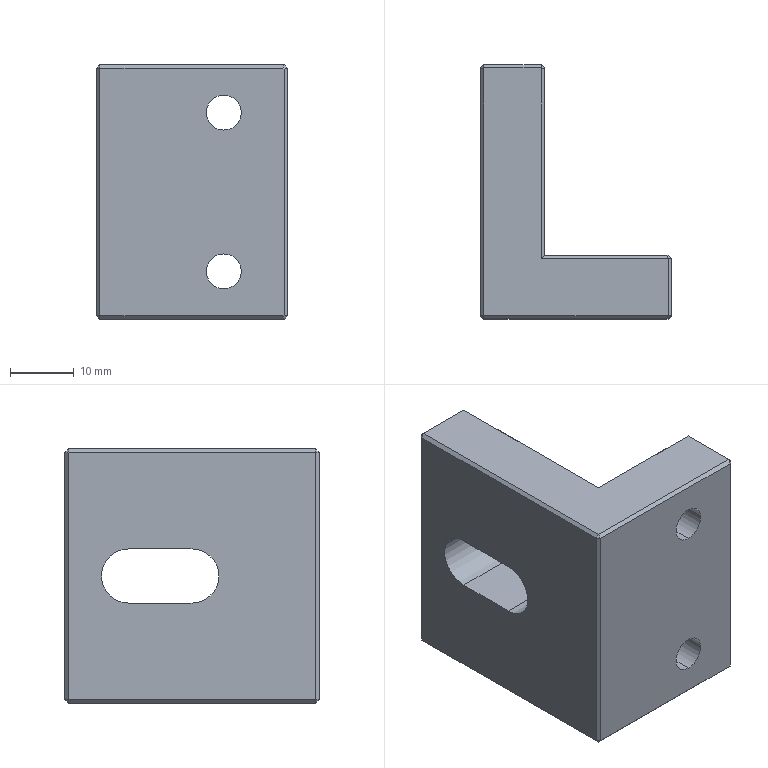Part | SolidWorks | features Chamfer 3, ICE 2, Extrusion 1, HoleWzd 1 | 1 solid | 49 faces | box 30 x 40 x 40 mm | volume 21456 mm3 | plane 39 | cylinder 10 | commonest cylinder face diameters 5.5 x4 10 x4 8.5 x2
STEP:
#1=CARTESIAN_POINT('',(5.,4.6,7.5));
#2=VERTEX_POINT('',#1);
#3=CARTESIAN_POINT('',(5.,4.6,17.5));
#4=VERTEX_POINT('',#3);
#5=CARTESIAN_POINT('',(5.,4.6,12.5));
#6=DIRECTION('',(0.,1.,0.));
#7=DIRECTION('',(0.,0.,1.));
#8=AXIS2_PLACEMENT_3D('',#5,#6,#7);
#9=CIRCLE('',#8,5.);
#10=EDGE_CURVE('',#2,#4,#9,.T.);
#11=ORIENTED_EDGE('',*,*,#10,.F.);
#12=CARTESIAN_POINT('',(5.,10.,7.5));
#13=VERTEX_POINT('',#12);
#14=CARTESIAN_POINT('',(5.,10.,7.5));
#15=DIRECTION('',(0.,1.,0.));
#16=VECTOR('',#15,1000.);
#17=LINE('',#14,#16);
#18=EDGE_CURVE('',#2,#13,#17,.T.);
#19=ORIENTED_EDGE('',*,*,#18,.T.);
#20=CARTESIAN_POINT('',(5.,10.,17.5));
#21=VERTEX_POINT('',#20);
#22=CARTESIAN_POINT('',(5.,10.,12.5));
#23=DIRECTION('',(0.,1.,0.));
#24=DIRECTION('',(0.,0.,1.));
#25=AXIS2_PLACEMENT_3D('',#22,#23,#24);
#26=CIRCLE('',#25,5.);
#27=EDGE_CURVE('',#13,#21,#26,.T.);
#28=ORIENTED_EDGE('',*,*,#27,.T.);
#29=CARTESIAN_POINT('',(5.,10.,17.5));
#30=DIRECTION('',(0.,1.,0.));
#31=VECTOR('',#30,1000.);
#32=LINE('',#29,#31);
#33=EDGE_CURVE('',#4,#21,#32,.T.);
#34=ORIENTED_EDGE('',*,*,#33,.F.);
#35=EDGE_LOOP('',(#11,#19,#28,#34));
#36=FACE_OUTER_BOUND('',#35,.T.);
#37=CARTESIAN_POINT('',(5.,10.,12.5));
#38=DIRECTION('',(0.,1.,0.));
#39=DIRECTION('',(0.,0.,1.));
#40=AXIS2_PLACEMENT_3D('',#37,#38,#39);
#41=CYLINDRICAL_SURFACE('',#40,5.);
#42=ADVANCED_FACE('',(#36),#41,.F.);
#43=CARTESIAN_POINT('',(5.,0.,9.75));
#44=VERTEX_POINT('',#43);
#45=CARTESIAN_POINT('',(5.,0.,15.25));
#46=VERTEX_POINT('',#45);
#47=CARTESIAN_POINT('',(5.,0.,12.5));
#48=DIRECTION('',(0.,1.,0.));
#49=DIRECTION('',(0.,0.,1.));
#50=AXIS2_PLACEMENT_3D('',#47,#48,#49);
#51=CIRCLE('',#50,2.75);
#52=EDGE_CURVE('',#44,#46,#51,.T.);
#53=ORIENTED_EDGE('',*,*,#52,.F.);
#54=CARTESIAN_POINT('',(5.,4.6,9.75));
#55=VERTEX_POINT('',#54);
#56=CARTESIAN_POINT('',(5.,10.,9.75));
#57=DIRECTION('',(0.,1.,0.));
#58=VECTOR('',#57,1000.);
#59=LINE('',#56,#58);
#60=EDGE_CURVE('',#44,#55,#59,.T.);
#61=ORIENTED_EDGE('',*,*,#60,.T.);
#62=CARTESIAN_POINT('',(5.,4.6,15.25));
#63=VERTEX_POINT('',#62);
#64=CARTESIAN_POINT('',(5.,4.6,12.5));
#65=DIRECTION('',(0.,1.,0.));
#66=DIRECTION('',(0.,0.,1.));
#67=AXIS2_PLACEMENT_3D('',#64,#65,#66);
#68=CIRCLE('',#67,2.75);
#69=EDGE_CURVE('',#55,#63,#68,.T.);
#70=ORIENTED_EDGE('',*,*,#69,.T.);
#71=CARTESIAN_POINT('',(5.,10.,15.25));
#72=DIRECTION('',(0.,1.,0.));
#73=VECTOR('',#72,1000.);
#74=LINE('',#71,#73);
#75=EDGE_CURVE('',#46,#63,#74,.T.);
#76=ORIENTED_EDGE('',*,*,#75,.F.);
#77=EDGE_LOOP('',(#53,#61,#70,#76));
#78=FACE_OUTER_BOUND('',#77,.T.);
#79=CARTESIAN_POINT('',(5.,10.,12.5));
#80=DIRECTION('',(0.,1.,0.));
#81=DIRECTION('',(0.,0.,1.));
#82=AXIS2_PLACEMENT_3D('',#79,#80,#81);
#83=CYLINDRICAL_SURFACE('',#82,2.75);
#84=ADVANCED_FACE('',(#78),#83,.F.);
#85=CARTESIAN_POINT('',(5.,4.6,-17.5));
#86=VERTEX_POINT('',#85);
#87=CARTESIAN_POINT('',(5.,4.6,-7.5));
#88=VERTEX_POINT('',#87);
#89=CARTESIAN_POINT('',(5.,4.6,-12.5));
#90=DIRECTION('',(0.,1.,0.));
#91=DIRECTION('',(0.,0.,1.));
#92=AXIS2_PLACEMENT_3D('',#89,#90,#91);
#93=CIRCLE('',#92,5.);
#94=EDGE_CURVE('',#86,#88,#93,.T.);
#95=ORIENTED_EDGE('',*,*,#94,.F.);
#96=CARTESIAN_POINT('',(5.,10.,-17.5));
#97=VERTEX_POINT('',#96);
#98=CARTESIAN_POINT('',(5.,10.,-17.5));
#99=DIRECTION('',(0.,1.,0.));
#100=VECTOR('',#99,1000.);
#101=LINE('',#98,#100);
#102=EDGE_CURVE('',#86,#97,#101,.T.);
#103=ORIENTED_EDGE('',*,*,#102,.T.);
#104=CARTESIAN_POINT('',(5.,10.,-7.5));
#105=VERTEX_POINT('',#104);
#106=CARTESIAN_POINT('',(5.,10.,-12.5));
#107=DIRECTION('',(0.,1.,0.));
#108=DIRECTION('',(0.,0.,1.));
#109=AXIS2_PLACEMENT_3D('',#106,#107,#108);
#110=CIRCLE('',#109,5.);
#111=EDGE_CURVE('',#97,#105,#110,.T.);
#112=ORIENTED_EDGE('',*,*,#111,.T.);
#113=CARTESIAN_POINT('',(5.,10.,-7.5));
#114=DIRECTION('',(0.,1.,0.));
#115=VECTOR('',#114,1000.);
#116=LINE('',#113,#115);
#117=EDGE_CURVE('',#88,#105,#116,.T.);
#118=ORIENTED_EDGE('',*,*,#117,.F.);
#119=EDGE_LOOP('',(#95,#103,#112,#118));
#120=FACE_OUTER_BOUND('',#119,.T.);
#121=CARTESIAN_POINT('',(5.,10.,-12.5));
#122=DIRECTION('',(0.,1.,0.));
#123=DIRECTION('',(0.,0.,1.));
#124=AXIS2_PLACEMENT_3D('',#121,#122,#123);
#125=CYLINDRICAL_SURFACE('',#124,5.);
#126=ADVANCED_FACE('',(#120),#125,.F.);
#127=CARTESIAN_POINT('',(5.,0.,-15.25));
#128=VERTEX_POINT('',#127);
#129=CARTESIAN_POINT('',(5.,0.,-9.75));
#130=VERTEX_POINT('',#129);
#131=CARTESIAN_POINT('',(5.,0.,-12.5));
#132=DIRECTION('',(0.,1.,0.));
#133=DIRECTION('',(0.,0.,1.));
#134=AXIS2_PLACEMENT_3D('',#131,#132,#133);
#135=CIRCLE('',#134,2.75);
#136=EDGE_CURVE('',#128,#130,#135,.T.);
#137=ORIENTED_EDGE('',*,*,#136,.F.);
#138=CARTESIAN_POINT('',(5.,4.6,-15.25));
#139=VERTEX_POINT('',#138);
#140=CARTESIAN_POINT('',(5.,10.,-15.25));
#141=DIRECTION('',(0.,1.,0.));
#142=VECTOR('',#141,1000.);
#143=LINE('',#140,#142);
#144=EDGE_CURVE('',#128,#139,#143,.T.);
#145=ORIENTED_EDGE('',*,*,#144,.T.);
#146=CARTESIAN_POINT('',(5.,4.6,-9.75));
#147=VERTEX_POINT('',#146);
#148=CARTESIAN_POINT('',(5.,4.6,-12.5));
#149=DIRECTION('',(0.,1.,0.));
#150=DIRECTION('',(0.,0.,1.));
#151=AXIS2_PLACEMENT_3D('',#148,#149,#150);
#152=CIRCLE('',#151,2.75);
#153=EDGE_CURVE('',#139,#147,#152,.T.);
#154=ORIENTED_EDGE('',*,*,#153,.T.);
#155=CARTESIAN_POINT('',(5.,10.,-9.75));
#156=DIRECTION('',(0.,1.,0.));
#157=VECTOR('',#156,1000.);
#158=LINE('',#155,#157);
#159=EDGE_CURVE('',#130,#147,#158,.T.);
#160=ORIENTED_EDGE('',*,*,#159,.F.);
#161=EDGE_LOOP('',(#137,#145,#154,#160));
#162=FACE_OUTER_BOUND('',#161,.T.);
#163=CARTESIAN_POINT('',(5.,10.,-12.5));
#164=DIRECTION('',(0.,1.,0.));
#165=DIRECTION('',(0.,0.,1.));
#166=AXIS2_PLACEMENT_3D('',#163,#164,#165);
#167=CYLINDRICAL_SURFACE('',#166,2.75);
#168=ADVANCED_FACE('',(#162),#167,.F.);
#169=CARTESIAN_POINT('',(15.,9.5,19.5));
#170=VERTEX_POINT('',#169);
#171=CARTESIAN_POINT('',(15.,0.5,19.5));
#172=VERTEX_POINT('',#171);
#173=CARTESIAN_POINT('',(15.,10.,19.5));
#174=DIRECTION('',(0.,-1.,0.));
#175=VECTOR('',#174,1000.);
#176=LINE('',#173,#175);
#177=EDGE_CURVE('',#170,#172,#176,.T.);
#178=ORIENTED_EDGE('',*,*,#177,.T.);
#179=CARTESIAN_POINT('',(15.,0.5,-19.5));
#180=VERTEX_POINT('',#179);
#181=CARTESIAN_POINT('',(15.,0.5,-20.));
#182=DIRECTION('',(0.,0.,-1.));
#183=VECTOR('',#182,1000.);
#184=LINE('',#181,#183);
#185=EDGE_CURVE('',#172,#180,#184,.T.);
#186=ORIENTED_EDGE('',*,*,#185,.T.);
#187=CARTESIAN_POINT('',(15.,9.5,-19.5));
#188=VERTEX_POINT('',#187);
#189=CARTESIAN_POINT('',(15.,10.,-19.5));
#190=DIRECTION('',(0.,1.,0.));
#191=VECTOR('',#190,1000.);
#192=LINE('',#189,#191);
#193=EDGE_CURVE('',#180,#188,#192,.T.);
#194=ORIENTED_EDGE('',*,*,#193,.T.);
#195=CARTESIAN_POINT('',(15.,9.5,19.5));
#196=DIRECTION('',(0.,0.,1.));
#197=VECTOR('',#196,1000.);
#198=LINE('',#195,#197);
#199=EDGE_CURVE('',#188,#170,#198,.T.);
#200=ORIENTED_EDGE('',*,*,#199,.T.);
#201=EDGE_LOOP('',(#178,#186,#194,#200));
#202=FACE_OUTER_BOUND('',#201,.T.);
#203=CARTESIAN_POINT('',(15.,10.,-20.));
#204=DIRECTION('',(-1.,0.,0.));
#205=DIRECTION('',(0.,0.,1.));
#206=AXIS2_PLACEMENT_3D('',#203,#204,#205);
#207=PLANE('',#206);
#208=ADVANCED_FACE('',(#202),#207,.F.);
#209=CARTESIAN_POINT('',(14.5,0.5,-20.));
#210=VERTEX_POINT('',#209);
#211=CARTESIAN_POINT('',(-14.5,0.5,-20.));
#212=VERTEX_POINT('',#211);
#213=CARTESIAN_POINT('',(-15.,0.5,-20.));
#214=DIRECTION('',(-1.,0.,0.));
#215=VECTOR('',#214,1000.);
#216=LINE('',#213,#215);
#217=EDGE_CURVE('',#210,#212,#216,.T.);
#218=ORIENTED_EDGE('',*,*,#217,.T.);
#219=CARTESIAN_POINT('',(-14.5,39.5,-20.));
#220=VERTEX_POINT('',#219);
#221=CARTESIAN_POINT('',(-14.5,10.,-20.));
#222=DIRECTION('',(0.,1.,0.));
#223=VECTOR('',#222,1000.);
#224=LINE('',#221,#223);
#225=EDGE_CURVE('',#212,#220,#224,.T.);
#226=ORIENTED_EDGE('',*,*,#225,.T.);
#227=CARTESIAN_POINT('',(-5.5,39.5,-20.));
#228=VERTEX_POINT('',#227);
#229=CARTESIAN_POINT('',(-5.,39.5,-20.));
#230=DIRECTION('',(1.,0.,0.));
#231=VECTOR('',#230,1000.);
#232=LINE('',#229,#231);
#233=EDGE_CURVE('',#220,#228,#232,.T.);
#234=ORIENTED_EDGE('',*,*,#233,.T.);
#235=CARTESIAN_POINT('',(-5.5,9.5,-20.));
#236=VERTEX_POINT('',#235);
#237=CARTESIAN_POINT('',(-5.5,10.,-20.));
#238=DIRECTION('',(0.,-1.,0.));
#239=VECTOR('',#238,1000.);
#240=LINE('',#237,#239);
#241=EDGE_CURVE('',#228,#236,#240,.T.);
#242=ORIENTED_EDGE('',*,*,#241,.T.);
#243=CARTESIAN_POINT('',(14.5,9.5,-20.));
#244=VERTEX_POINT('',#243);
#245=CARTESIAN_POINT('',(14.5,9.5,-20.));
#246=DIRECTION('',(1.,0.,0.));
#247=VECTOR('',#246,1000.);
#248=LINE('',#245,#247);
#249=EDGE_CURVE('',#236,#244,#248,.T.);
#250=ORIENTED_EDGE('',*,*,#249,.T.);
#251=CARTESIAN_POINT('',(14.5,10.,-20.));
#252=DIRECTION('',(0.,-1.,0.));
#253=VECTOR('',#252,1000.);
#254=LINE('',#251,#253);
#255=EDGE_CURVE('',#244,#210,#254,.T.);
#256=ORIENTED_EDGE('',*,*,#255,.T.);
#257=EDGE_LOOP('',(#218,#226,#234,#242,#250,#256));
#258=FACE_OUTER_BOUND('',#257,.T.);
#259=CARTESIAN_POINT('',(-15.,10.,-20.));
#260=DIRECTION('',(0.,0.,1.));
#261=DIRECTION('',(1.,0.,0.));
#262=AXIS2_PLACEMENT_3D('',#259,#260,#261);
#263=PLANE('',#262);
#264=ADVANCED_FACE('',(#258),#263,.F.);
#265=CARTESIAN_POINT('',(-15.,0.5,-19.5));
#266=VERTEX_POINT('',#265);
#267=CARTESIAN_POINT('',(-15.,0.5,19.5));
#268=VERTEX_POINT('',#267);
#269=CARTESIAN_POINT('',(-15.,0.5,-20.));
#270=DIRECTION('',(0.,0.,1.));
#271=VECTOR('',#270,1000.);
#272=LINE('',#269,#271);
#273=EDGE_CURVE('',#266,#268,#272,.T.);
#274=ORIENTED_EDGE('',*,*,#273,.T.);
#275=CARTESIAN_POINT('',(-15.,39.293,19.5));
#276=VERTEX_POINT('',#275);
#277=CARTESIAN_POINT('',(-15.,10.,19.5));
#278=DIRECTION('',(0.,1.,0.));
#279=VECTOR('',#278,1000.);
#280=LINE('',#277,#279);
#281=EDGE_CURVE('',#268,#276,#280,.T.);
#282=ORIENTED_EDGE('',*,*,#281,.T.);
#283=CARTESIAN_POINT('',(-15.,39.5,19.293));
#284=VERTEX_POINT('',#283);
#285=CARTESIAN_POINT('',(-15.,39.646,19.146));
#286=DIRECTION('',(0.,0.7071,-0.7071));
#287=VECTOR('',#286,1000.);
#288=LINE('',#285,#287);
#289=EDGE_CURVE('',#276,#284,#288,.T.);
#290=ORIENTED_EDGE('',*,*,#289,.T.);
#291=CARTESIAN_POINT('',(-15.,39.5,-19.293));
#292=VERTEX_POINT('',#291);
#293=CARTESIAN_POINT('',(-15.,39.5,-19.5));
#294=DIRECTION('',(0.,0.,-1.));
#295=VECTOR('',#294,1000.);
#296=LINE('',#293,#295);
#297=EDGE_CURVE('',#284,#292,#296,.T.);
#298=ORIENTED_EDGE('',*,*,#297,.T.);
#299=CARTESIAN_POINT('',(-15.,39.293,-19.5));
#300=VERTEX_POINT('',#299);
#301=CARTESIAN_POINT('',(-15.,39.146,-19.646));
#302=DIRECTION('',(0.,-0.7071,-0.7071));
#303=VECTOR('',#302,1000.);
#304=LINE('',#301,#303);
#305=EDGE_CURVE('',#292,#300,#304,.T.);
#306=ORIENTED_EDGE('',*,*,#305,.T.);
#307=CARTESIAN_POINT('',(-15.,10.,-19.5));
#308=DIRECTION('',(0.,-1.,0.));
#309=VECTOR('',#308,1000.);
#310=LINE('',#307,#309);
#311=EDGE_CURVE('',#300,#266,#310,.T.);
#312=ORIENTED_EDGE('',*,*,#311,.T.);
#313=EDGE_LOOP('',(#274,#282,#290,#298,#306,#312));
#314=FACE_OUTER_BOUND('',#313,.T.);
#315=CARTESIAN_POINT('',(-15.,20.,-4.25));
#316=VERTEX_POINT('',#315);
#317=CARTESIAN_POINT('',(-15.,30.,-4.25));
#318=VERTEX_POINT('',#317);
#319=CARTESIAN_POINT('',(-15.,30.,-4.25));
#320=DIRECTION('',(0.,1.,0.));
#321=VECTOR('',#320,1000.);
#322=LINE('',#319,#321);
#323=EDGE_CURVE('',#316,#318,#322,.T.);
#324=ORIENTED_EDGE('',*,*,#323,.T.);
#325=CARTESIAN_POINT('',(-15.,30.,4.25));
#326=VERTEX_POINT('',#325);
#327=CARTESIAN_POINT('',(-15.,30.,0.));
#328=DIRECTION('',(1.,0.,0.));
#329=DIRECTION('',(0.,0.,-1.));
#330=AXIS2_PLACEMENT_3D('',#327,#328,#329);
#331=CIRCLE('',#330,4.25);
#332=EDGE_CURVE('',#318,#326,#331,.T.);
#333=ORIENTED_EDGE('',*,*,#332,.T.);
#334=CARTESIAN_POINT('',(-15.,20.,4.25));
#335=VERTEX_POINT('',#334);
#336=CARTESIAN_POINT('',(-15.,30.,4.25));
#337=DIRECTION('',(0.,-1.,0.));
#338=VECTOR('',#337,1000.);
#339=LINE('',#336,#338);
#340=EDGE_CURVE('',#326,#335,#339,.T.);
#341=ORIENTED_EDGE('',*,*,#340,.T.);
#342=CARTESIAN_POINT('',(-15.,20.,0.));
#343=DIRECTION('',(1.,0.,0.));
#344=DIRECTION('',(0.,0.,-1.));
#345=AXIS2_PLACEMENT_3D('',#342,#343,#344);
#346=CIRCLE('',#345,4.25);
#347=EDGE_CURVE('',#335,#316,#346,.T.);
#348=ORIENTED_EDGE('',*,*,#347,.T.);
#349=EDGE_LOOP('',(#324,#333,#341,#348));
#350=FACE_BOUND('',#349,.T.);
#351=CARTESIAN_POINT('',(-15.,10.,-20.));
#352=DIRECTION('',(1.,0.,0.));
#353=DIRECTION('',(0.,0.,-1.));
#354=AXIS2_PLACEMENT_3D('',#351,#352,#353);
#355=PLANE('',#354);
#356=ADVANCED_FACE('',(#314,#350),#355,.F.);
#357=CARTESIAN_POINT('',(-5.5,39.5,20.));
#358=VERTEX_POINT('',#357);
#359=CARTESIAN_POINT('',(-14.5,39.5,20.));
#360=VERTEX_POINT('',#359);
#361=CARTESIAN_POINT('',(-15.,39.5,20.));
#362=DIRECTION('',(-1.,0.,0.));
#363=VECTOR('',#362,1000.);
#364=LINE('',#361,#363);
#365=EDGE_CURVE('',#358,#360,#364,.T.);
#366=ORIENTED_EDGE('',*,*,#365,.T.);
#367=CARTESIAN_POINT('',(-14.5,0.5,20.));
#368=VERTEX_POINT('',#367);
#369=CARTESIAN_POINT('',(-14.5,10.,20.));
#370=DIRECTION('',(0.,-1.,0.));
#371=VECTOR('',#370,1000.);
#372=LINE('',#369,#371);
#373=EDGE_CURVE('',#360,#368,#372,.T.);
#374=ORIENTED_EDGE('',*,*,#373,.T.);
#375=CARTESIAN_POINT('',(14.5,0.5,20.));
#376=VERTEX_POINT('',#375);
#377=CARTESIAN_POINT('',(-15.,0.5,20.));
#378=DIRECTION('',(1.,0.,0.));
#379=VECTOR('',#378,1000.);
#380=LINE('',#377,#379);
#381=EDGE_CURVE('',#368,#376,#380,.T.);
#382=ORIENTED_EDGE('',*,*,#381,.T.);
#383=CARTESIAN_POINT('',(14.5,9.5,20.));
#384=VERTEX_POINT('',#383);
#385=CARTESIAN_POINT('',(14.5,10.,20.));
#386=DIRECTION('',(0.,1.,0.));
#387=VECTOR('',#386,1000.);
#388=LINE('',#385,#387);
#389=EDGE_CURVE('',#376,#384,#388,.T.);
#390=ORIENTED_EDGE('',*,*,#389,.T.);
#391=CARTESIAN_POINT('',(-5.5,9.5,20.));
#392=VERTEX_POINT('',#391);
#393=CARTESIAN_POINT('',(-5.,9.5,20.));
#394=DIRECTION('',(-1.,0.,0.));
#395=VECTOR('',#394,1000.);
#396=LINE('',#393,#395);
#397=EDGE_CURVE('',#384,#392,#396,.T.);
#398=ORIENTED_EDGE('',*,*,#397,.T.);
#399=CARTESIAN_POINT('',(-5.5,39.5,20.));
#400=DIRECTION('',(0.,1.,0.));
#401=VECTOR('',#400,1000.);
#402=LINE('',#399,#401);
#403=EDGE_CURVE('',#392,#358,#402,.T.);
#404=ORIENTED_EDGE('',*,*,#403,.T.);
#405=EDGE_LOOP('',(#366,#374,#382,#390,#398,#404));
#406=FACE_OUTER_BOUND('',#405,.T.);
#407=CARTESIAN_POINT('',(-15.,10.,20.));
#408=DIRECTION('',(0.,0.,-1.));
#409=DIRECTION('',(-1.,0.,0.));
#410=AXIS2_PLACEMENT_3D('',#407,#408,#409);
#411=PLANE('',#410);
#412=ADVANCED_FACE('',(#406),#411,.F.);
#413=CARTESIAN_POINT('',(-5.,10.,19.5));
#414=VERTEX_POINT('',#413);
#415=CARTESIAN_POINT('',(-5.,10.,-19.5));
#416=VERTEX_POINT('',#415);
#417=CARTESIAN_POINT('',(-5.,10.,0.));
#418=DIRECTION('',(0.,0.,-1.));
#419=VECTOR('',#418,1000.);
#420=LINE('',#417,#419);
#421=EDGE_CURVE('',#414,#416,#420,.T.);
#422=ORIENTED_EDGE('',*,*,#421,.F.);
#423=CARTESIAN_POINT('',(14.293,10.,19.5));
#424=VERTEX_POINT('',#423);
#425=CARTESIAN_POINT('',(14.5,10.,19.5));
#426=DIRECTION('',(1.,0.,0.));
#427=VECTOR('',#426,1000.);
#428=LINE('',#425,#427);
#429=EDGE_CURVE('',#414,#424,#428,.T.);
#430=ORIENTED_EDGE('',*,*,#429,.T.);
#431=CARTESIAN_POINT('',(14.5,10.,19.293));
#432=VERTEX_POINT('',#431);
#433=CARTESIAN_POINT('',(16.896,10.,16.896));
#434=DIRECTION('',(0.7071,0.,-0.7071));
#435=VECTOR('',#434,1000.);
#436=LINE('',#433,#435);
#437=EDGE_CURVE('',#424,#432,#436,.T.);
#438=ORIENTED_EDGE('',*,*,#437,.T.);
#439=CARTESIAN_POINT('',(14.5,10.,-19.293));
#440=VERTEX_POINT('',#439);
#441=CARTESIAN_POINT('',(14.5,10.,-19.5));
#442=DIRECTION('',(0.,0.,-1.));
#443=VECTOR('',#442,1000.);
#444=LINE('',#441,#443);
#445=EDGE_CURVE('',#432,#440,#444,.T.);
#446=ORIENTED_EDGE('',*,*,#445,.T.);
#447=CARTESIAN_POINT('',(14.293,10.,-19.5));
#448=VERTEX_POINT('',#447);
#449=CARTESIAN_POINT('',(16.896,10.,-16.896));
#450=DIRECTION('',(-0.7071,0.,-0.7071));
#451=VECTOR('',#450,1000.);
#452=LINE('',#449,#451);
#453=EDGE_CURVE('',#440,#448,#452,.T.);
#454=ORIENTED_EDGE('',*,*,#453,.T.);
#455=CARTESIAN_POINT('',(-5.,10.,-19.5));
#456=DIRECTION('',(-1.,0.,0.));
#457=VECTOR('',#456,1000.);
#458=LINE('',#455,#457);
#459=EDGE_CURVE('',#448,#416,#458,.T.);
#460=ORIENTED_EDGE('',*,*,#459,.T.);
#461=EDGE_LOOP('',(#422,#430,#438,#446,#454,#460));
#462=FACE_OUTER_BOUND('',#461,.T.);
#463=CARTESIAN_POINT('',(5.,10.,12.5));
#464=DIRECTION('',(0.,1.,0.));
#465=DIRECTION('',(0.,0.,1.));
#466=AXIS2_PLACEMENT_3D('',#463,#464,#465);
#467=CIRCLE('',#466,5.);
#468=EDGE_CURVE('',#21,#13,#467,.T.);
#469=ORIENTED_EDGE('',*,*,#468,.F.);
#470=ORIENTED_EDGE('',*,*,#27,.F.);
#471=EDGE_LOOP('',(#469,#470));
#472=FACE_BOUND('',#471,.T.);
#473=CARTESIAN_POINT('',(5.,10.,-12.5));
#474=DIRECTION('',(0.,1.,0.));
#475=DIRECTION('',(0.,0.,1.));
#476=AXIS2_PLACEMENT_3D('',#473,#474,#475);
#477=CIRCLE('',#476,5.);
#478=EDGE_CURVE('',#105,#97,#477,.T.);
#479=ORIENTED_EDGE('',*,*,#478,.F.);
#480=ORIENTED_EDGE('',*,*,#111,.F.);
#481=EDGE_LOOP('',(#479,#480));
#482=FACE_BOUND('',#481,.T.);
#483=CARTESIAN_POINT('',(0.,10.,0.));
#484=DIRECTION('',(0.,1.,0.));
#485=DIRECTION('',(0.,0.,1.));
#486=AXIS2_PLACEMENT_3D('',#483,#484,#485);
#487=PLANE('',#486);
#488=ADVANCED_FACE('',(#462,#472,#482),#487,.T.);
#489=CARTESIAN_POINT('',(14.293,0.,19.5));
#490=VERTEX_POINT('',#489);
#491=CARTESIAN_POINT('',(-14.5,0.,19.5));
#492=VERTEX_POINT('',#491);
#493=CARTESIAN_POINT('',(0.,0.,19.5));
#494=DIRECTION('',(-1.,0.,0.));
#495=VECTOR('',#494,1000.);
#496=LINE('',#493,#495);
#497=EDGE_CURVE('',#490,#492,#496,.T.);
#498=ORIENTED_EDGE('',*,*,#497,.T.);
#499=CARTESIAN_POINT('',(-14.5,0.,-19.5));
#500=VERTEX_POINT('',#499);
#501=CARTESIAN_POINT('',(-14.5,0.,0.));
#502=DIRECTION('',(0.,0.,-1.));
#503=VECTOR('',#502,1000.);
#504=LINE('',#501,#503);
#505=EDGE_CURVE('',#492,#500,#504,.T.);
#506=ORIENTED_EDGE('',*,*,#505,.T.);
#507=CARTESIAN_POINT('',(14.293,0.,-19.5));
#508=VERTEX_POINT('',#507);
#509=CARTESIAN_POINT('',(0.,0.,-19.5));
#510=DIRECTION('',(1.,0.,0.));
#511=VECTOR('',#510,1000.);
#512=LINE('',#509,#511);
#513=EDGE_CURVE('',#500,#508,#512,.T.);
#514=ORIENTED_EDGE('',*,*,#513,.T.);
#515=CARTESIAN_POINT('',(14.5,0.,-19.293));
#516=VERTEX_POINT('',#515);
#517=CARTESIAN_POINT('',(14.646,0.,-19.146));
#518=DIRECTION('',(0.7071,0.,0.7071));
#519=VECTOR('',#518,1000.);
#520=LINE('',#517,#519);
#521=EDGE_CURVE('',#508,#516,#520,.T.);
#522=ORIENTED_EDGE('',*,*,#521,.T.);
#523=CARTESIAN_POINT('',(14.5,0.,19.293));
#524=VERTEX_POINT('',#523);
#525=CARTESIAN_POINT('',(14.5,0.,0.));
#526=DIRECTION('',(0.,0.,1.));
#527=VECTOR('',#526,1000.);
#528=LINE('',#525,#527);
#529=EDGE_CURVE('',#516,#524,#528,.T.);
#530=ORIENTED_EDGE('',*,*,#529,.T.);
#531=CARTESIAN_POINT('',(14.146,0.,19.646));
#532=DIRECTION('',(-0.7071,0.,0.7071));
#533=VECTOR('',#532,1000.);
#534=LINE('',#531,#533);
#535=EDGE_CURVE('',#524,#490,#534,.T.);
#536=ORIENTED_EDGE('',*,*,#535,.T.);
#537=EDGE_LOOP('',(#498,#506,#514,#522,#530,#536));
#538=FACE_OUTER_BOUND('',#537,.T.);
#539=CARTESIAN_POINT('',(5.,0.,12.5));
#540=DIRECTION('',(0.,1.,0.));
#541=DIRECTION('',(0.,0.,1.));
#542=AXIS2_PLACEMENT_3D('',#539,#540,#541);
#543=CIRCLE('',#542,2.75);
#544=EDGE_CURVE('',#46,#44,#543,.T.);
#545=ORIENTED_EDGE('',*,*,#544,.T.);
#546=ORIENTED_EDGE('',*,*,#52,.T.);
#547=EDGE_LOOP('',(#545,#546));
#548=FACE_BOUND('',#547,.T.);
#549=CARTESIAN_POINT('',(5.,0.,-12.5));
#550=DIRECTION('',(0.,1.,0.));
#551=DIRECTION('',(0.,0.,1.));
#552=AXIS2_PLACEMENT_3D('',#549,#550,#551);
#553=CIRCLE('',#552,2.75);
#554=EDGE_CURVE('',#130,#128,#553,.T.);
#555=ORIENTED_EDGE('',*,*,#554,.T.);
#556=ORIENTED_EDGE('',*,*,#136,.T.);
#557=EDGE_LOOP('',(#555,#556));
#558=FACE_BOUND('',#557,.T.);
#559=CARTESIAN_POINT('',(0.,0.,0.));
#560=DIRECTION('',(0.,1.,0.));
#561=DIRECTION('',(0.,0.,1.));
#562=AXIS2_PLACEMENT_3D('',#559,#560,#561);
#563=PLANE('',#562);
#564=ADVANCED_FACE('',(#538,#548,#558),#563,.F.);
#565=CARTESIAN_POINT('',(-5.5,40.,-19.5));
#566=VERTEX_POINT('',#565);
#567=CARTESIAN_POINT('',(-14.5,40.,-19.5));
#568=VERTEX_POINT('',#567);
#569=CARTESIAN_POINT('',(-15.,40.,-19.5));
#570=DIRECTION('',(-1.,0.,0.));
#571=VECTOR('',#570,1000.);
#572=LINE('',#569,#571);
#573=EDGE_CURVE('',#566,#568,#572,.T.);
#574=ORIENTED_EDGE('',*,*,#573,.T.);
#575=CARTESIAN_POINT('',(-14.5,40.,19.5));
#576=VERTEX_POINT('',#575);
#577=CARTESIAN_POINT('',(-14.5,40.,19.5));
#578=DIRECTION('',(0.,0.,1.));
#579=VECTOR('',#578,1000.);
#580=LINE('',#577,#579);
#581=EDGE_CURVE('',#568,#576,#580,.T.);
#582=ORIENTED_EDGE('',*,*,#581,.T.);
#583=CARTESIAN_POINT('',(-5.5,40.,19.5));
#584=VERTEX_POINT('',#583);
#585=CARTESIAN_POINT('',(-5.,40.,19.5));
#586=DIRECTION('',(1.,0.,0.));
#587=VECTOR('',#586,1000.);
#588=LINE('',#585,#587);
#589=EDGE_CURVE('',#576,#584,#588,.T.);
#590=ORIENTED_EDGE('',*,*,#589,.T.);
#591=CARTESIAN_POINT('',(-5.5,40.,-20.));
#592=DIRECTION('',(0.,0.,-1.));
#593=VECTOR('',#592,1000.);
#594=LINE('',#591,#593);
#595=EDGE_CURVE('',#584,#566,#594,.T.);
#596=ORIENTED_EDGE('',*,*,#595,.T.);
#597=EDGE_LOOP('',(#574,#582,#590,#596));
#598=FACE_OUTER_BOUND('',#597,.T.);
#599=CARTESIAN_POINT('',(-5.,40.,-20.));
#600=DIRECTION('',(0.,1.,0.));
#601=DIRECTION('',(0.,0.,1.));
#602=AXIS2_PLACEMENT_3D('',#599,#600,#601);
#603=PLANE('',#602);
#604=ADVANCED_FACE('',(#598),#603,.T.);
#605=CARTESIAN_POINT('',(-5.,30.,-4.25));
#606=VERTEX_POINT('',#605);
#607=CARTESIAN_POINT('',(-5.,30.,4.25));
#608=VERTEX_POINT('',#607);
#609=CARTESIAN_POINT('',(-5.,30.,0.));
#610=DIRECTION('',(1.,0.,0.));
#611=DIRECTION('',(0.,0.,-1.));
#612=AXIS2_PLACEMENT_3D('',#609,#610,#611);
#613=CIRCLE('',#612,4.25);
#614=EDGE_CURVE('',#606,#608,#613,.T.);
#615=ORIENTED_EDGE('',*,*,#614,.F.);
#616=CARTESIAN_POINT('',(-5.,20.,-4.25));
#617=VERTEX_POINT('',#616);
#618=CARTESIAN_POINT('',(-5.,30.,-4.25));
#619=DIRECTION('',(0.,1.,0.));
#620=VECTOR('',#619,1000.);
#621=LINE('',#618,#620);
#622=EDGE_CURVE('',#617,#606,#621,.T.);
#623=ORIENTED_EDGE('',*,*,#622,.F.);
#624=CARTESIAN_POINT('',(-5.,20.,4.25));
#625=VERTEX_POINT('',#624);
#626=CARTESIAN_POINT('',(-5.,20.,0.));
#627=DIRECTION('',(1.,0.,0.));
#628=DIRECTION('',(0.,0.,-1.));
#629=AXIS2_PLACEMENT_3D('',#626,#627,#628);
#630=CIRCLE('',#629,4.25);
#631=EDGE_CURVE('',#625,#617,#630,.T.);
#632=ORIENTED_EDGE('',*,*,#631,.F.);
#633=CARTESIAN_POINT('',(-5.,30.,4.25));
#634=DIRECTION('',(0.,-1.,0.));
#635=VECTOR('',#634,1000.);
#636=LINE('',#633,#635);
#637=EDGE_CURVE('',#608,#625,#636,.T.);
#638=ORIENTED_EDGE('',*,*,#637,.F.);
#639=EDGE_LOOP('',(#615,#623,#632,#638));
#640=FACE_BOUND('',#639,.T.);
#641=CARTESIAN_POINT('',(-5.,39.5,19.293));
#642=VERTEX_POINT('',#641);
#643=CARTESIAN_POINT('',(-5.,39.293,19.5));
#644=VERTEX_POINT('',#643);
#645=CARTESIAN_POINT('',(-5.,29.396,29.396));
#646=DIRECTION('',(0.,-0.7071,0.7071));
#647=VECTOR('',#646,1000.);
#648=LINE('',#645,#647);
#649=EDGE_CURVE('',#642,#644,#648,.T.);
#650=ORIENTED_EDGE('',*,*,#649,.T.);
#651=CARTESIAN_POINT('',(-5.,10.,19.5));
#652=DIRECTION('',(0.,-1.,0.));
#653=VECTOR('',#652,1000.);
#654=LINE('',#651,#653);
#655=EDGE_CURVE('',#644,#414,#654,.T.);
#656=ORIENTED_EDGE('',*,*,#655,.T.);
#657=ORIENTED_EDGE('',*,*,#421,.T.);
#658=CARTESIAN_POINT('',(-5.,39.293,-19.5));
#659=VERTEX_POINT('',#658);
#660=CARTESIAN_POINT('',(-5.,39.5,-19.5));
#661=DIRECTION('',(0.,1.,0.));
#662=VECTOR('',#661,1000.);
#663=LINE('',#660,#662);
#664=EDGE_CURVE('',#416,#659,#663,.T.);
#665=ORIENTED_EDGE('',*,*,#664,.T.);
#666=CARTESIAN_POINT('',(-5.,39.5,-19.293));
#667=VERTEX_POINT('',#666);
#668=CARTESIAN_POINT('',(-5.,29.396,-29.396));
#669=DIRECTION('',(0.,0.7071,0.7071));
#670=VECTOR('',#669,1000.);
#671=LINE('',#668,#670);
#672=EDGE_CURVE('',#659,#667,#671,.T.);
#673=ORIENTED_EDGE('',*,*,#672,.T.);
#674=CARTESIAN_POINT('',(-5.,39.5,0.));
#675=DIRECTION('',(0.,0.,1.));
#676=VECTOR('',#675,1000.);
#677=LINE('',#674,#676);
#678=EDGE_CURVE('',#667,#642,#677,.T.);
#679=ORIENTED_EDGE('',*,*,#678,.T.);
#680=EDGE_LOOP('',(#650,#656,#657,#665,#673,#679));
#681=FACE_OUTER_BOUND('',#680,.T.);
#682=CARTESIAN_POINT('',(-5.,0.,0.));
#683=DIRECTION('',(1.,0.,0.));
#684=DIRECTION('',(0.,0.,-1.));
#685=AXIS2_PLACEMENT_3D('',#682,#683,#684);
#686=PLANE('',#685);
#687=ADVANCED_FACE('',(#640,#681),#686,.T.);
#688=ORIENTED_EDGE('',*,*,#144,.F.);
#689=ORIENTED_EDGE('',*,*,#554,.F.);
#690=ORIENTED_EDGE('',*,*,#159,.T.);
#691=CARTESIAN_POINT('',(5.,4.6,-12.5));
#692=DIRECTION('',(0.,1.,0.));
#693=DIRECTION('',(0.,0.,1.));
#694=AXIS2_PLACEMENT_3D('',#691,#692,#693);
#695=CIRCLE('',#694,2.75);
#696=EDGE_CURVE('',#147,#139,#695,.T.);
#697=ORIENTED_EDGE('',*,*,#696,.T.);
#698=EDGE_LOOP('',(#688,#689,#690,#697));
#699=FACE_OUTER_BOUND('',#698,.T.);
#700=CARTESIAN_POINT('',(5.,10.,-12.5));
#701=DIRECTION('',(0.,1.,0.));
#702=DIRECTION('',(0.,0.,1.));
#703=AXIS2_PLACEMENT_3D('',#700,#701,#702);
#704=CYLINDRICAL_SURFACE('',#703,2.75);
#705=ADVANCED_FACE('',(#699),#704,.F.);
#706=ORIENTED_EDGE('',*,*,#696,.F.);
#707=ORIENTED_EDGE('',*,*,#153,.F.);
#708=EDGE_LOOP('',(#706,#707));
#709=FACE_BOUND('',#708,.T.);
#710=CARTESIAN_POINT('',(5.,4.6,-12.5));
#711=DIRECTION('',(0.,1.,0.));
#712=DIRECTION('',(0.,0.,1.));
#713=AXIS2_PLACEMENT_3D('',#710,#711,#712);
#714=CIRCLE('',#713,5.);
#715=EDGE_CURVE('',#88,#86,#714,.T.);
#716=ORIENTED_EDGE('',*,*,#715,.T.);
#717=ORIENTED_EDGE('',*,*,#94,.T.);
#718=EDGE_LOOP('',(#716,#717));
#719=FACE_OUTER_BOUND('',#718,.T.);
#720=CARTESIAN_POINT('',(7.75,4.6,-12.5));
#721=DIRECTION('',(0.,-1.,0.));
#722=DIRECTION('',(0.,0.,-1.));
#723=AXIS2_PLACEMENT_3D('',#720,#721,#722);
#724=PLANE('',#723);
#725=ADVANCED_FACE('',(#709,#719),#724,.F.);
#726=ORIENTED_EDGE('',*,*,#102,.F.);
#727=ORIENTED_EDGE('',*,*,#715,.F.);
#728=ORIENTED_EDGE('',*,*,#117,.T.);
#729=ORIENTED_EDGE('',*,*,#478,.T.);
#730=EDGE_LOOP('',(#726,#727,#728,#729));
#731=FACE_OUTER_BOUND('',#730,.T.);
#732=CARTESIAN_POINT('',(5.,10.,-12.5));
#733=DIRECTION('',(0.,1.,0.));
#734=DIRECTION('',(0.,0.,1.));
#735=AXIS2_PLACEMENT_3D('',#732,#733,#734);
#736=CYLINDRICAL_SURFACE('',#735,5.);
#737=ADVANCED_FACE('',(#731),#736,.F.);
#738=ORIENTED_EDGE('',*,*,#60,.F.);
#739=ORIENTED_EDGE('',*,*,#544,.F.);
#740=ORIENTED_EDGE('',*,*,#75,.T.);
#741=CARTESIAN_POINT('',(5.,4.6,12.5));
#742=DIRECTION('',(0.,1.,0.));
#743=DIRECTION('',(0.,0.,1.));
#744=AXIS2_PLACEMENT_3D('',#741,#742,#743);
#745=CIRCLE('',#744,2.75);
#746=EDGE_CURVE('',#63,#55,#745,.T.);
#747=ORIENTED_EDGE('',*,*,#746,.T.);
#748=EDGE_LOOP('',(#738,#739,#740,#747));
#749=FACE_OUTER_BOUND('',#748,.T.);
#750=CARTESIAN_POINT('',(5.,10.,12.5));
#751=DIRECTION('',(0.,1.,0.));
#752=DIRECTION('',(0.,0.,1.));
#753=AXIS2_PLACEMENT_3D('',#750,#751,#752);
#754=CYLINDRICAL_SURFACE('',#753,2.75);
#755=ADVANCED_FACE('',(#749),#754,.F.);
#756=ORIENTED_EDGE('',*,*,#746,.F.);
#757=ORIENTED_EDGE('',*,*,#69,.F.);
#758=EDGE_LOOP('',(#756,#757));
#759=FACE_BOUND('',#758,.T.);
#760=CARTESIAN_POINT('',(5.,4.6,12.5));
#761=DIRECTION('',(0.,1.,0.));
#762=DIRECTION('',(0.,0.,1.));
#763=AXIS2_PLACEMENT_3D('',#760,#761,#762);
#764=CIRCLE('',#763,5.);
#765=EDGE_CURVE('',#4,#2,#764,.T.);
#766=ORIENTED_EDGE('',*,*,#765,.T.);
#767=ORIENTED_EDGE('',*,*,#10,.T.);
#768=EDGE_LOOP('',(#766,#767));
#769=FACE_OUTER_BOUND('',#768,.T.);
#770=CARTESIAN_POINT('',(7.75,4.6,12.5));
#771=DIRECTION('',(0.,-1.,0.));
#772=DIRECTION('',(0.,0.,-1.));
#773=AXIS2_PLACEMENT_3D('',#770,#771,#772);
#774=PLANE('',#773);
#775=ADVANCED_FACE('',(#759,#769),#774,.F.);
#776=ORIENTED_EDGE('',*,*,#18,.F.);
#777=ORIENTED_EDGE('',*,*,#765,.F.);
#778=ORIENTED_EDGE('',*,*,#33,.T.);
#779=ORIENTED_EDGE('',*,*,#468,.T.);
#780=EDGE_LOOP('',(#776,#777,#778,#779));
#781=FACE_OUTER_BOUND('',#780,.T.);
#782=CARTESIAN_POINT('',(5.,10.,12.5));
#783=DIRECTION('',(0.,1.,0.));
#784=DIRECTION('',(0.,0.,1.));
#785=AXIS2_PLACEMENT_3D('',#782,#783,#784);
#786=CYLINDRICAL_SURFACE('',#785,5.);
#787=ADVANCED_FACE('',(#781),#786,.F.);
#788=ORIENTED_EDGE('',*,*,#193,.F.);
#789=CARTESIAN_POINT('',(14.5,0.5,-20.));
#790=DIRECTION('',(-0.7071,0.,-0.7071));
#791=VECTOR('',#790,1000.);
#792=LINE('',#789,#791);
#793=EDGE_CURVE('',#180,#210,#792,.T.);
#794=ORIENTED_EDGE('',*,*,#793,.T.);
#795=ORIENTED_EDGE('',*,*,#255,.F.);
#796=CARTESIAN_POINT('',(14.5,9.5,-20.));
#797=DIRECTION('',(0.7071,0.,0.7071));
#798=VECTOR('',#797,1000.);
#799=LINE('',#796,#798);
#800=EDGE_CURVE('',#244,#188,#799,.T.);
#801=ORIENTED_EDGE('',*,*,#800,.T.);
#802=EDGE_LOOP('',(#788,#794,#795,#801));
#803=FACE_OUTER_BOUND('',#802,.T.);
#804=CARTESIAN_POINT('',(14.5,10.,-20.));
#805=DIRECTION('',(-0.7071,0.,0.7071));
#806=DIRECTION('',(0.,-1.,0.));
#807=AXIS2_PLACEMENT_3D('',#804,#805,#806);
#808=PLANE('',#807);
#809=ADVANCED_FACE('',(#803),#808,.F.);
#810=ORIENTED_EDGE('',*,*,#389,.F.);
#811=CARTESIAN_POINT('',(15.,0.5,19.5));
#812=DIRECTION('',(0.7071,0.,-0.7071));
#813=VECTOR('',#812,1000.);
#814=LINE('',#811,#813);
#815=EDGE_CURVE('',#376,#172,#814,.T.);
#816=ORIENTED_EDGE('',*,*,#815,.T.);
#817=ORIENTED_EDGE('',*,*,#177,.F.);
#818=CARTESIAN_POINT('',(15.,9.5,19.5));
#819=DIRECTION('',(-0.7071,0.,0.7071));
#820=VECTOR('',#819,1000.);
#821=LINE('',#818,#820);
#822=EDGE_CURVE('',#170,#384,#821,.T.);
#823=ORIENTED_EDGE('',*,*,#822,.T.);
#824=EDGE_LOOP('',(#810,#816,#817,#823));
#825=FACE_OUTER_BOUND('',#824,.T.);
#826=CARTESIAN_POINT('',(15.,10.,19.5));
#827=DIRECTION('',(-0.7071,0.,-0.7071));
#828=DIRECTION('',(0.,-1.,0.));
#829=AXIS2_PLACEMENT_3D('',#826,#827,#828);
#830=PLANE('',#829);
#831=ADVANCED_FACE('',(#825),#830,.F.);
#832=ORIENTED_EDGE('',*,*,#614,.T.);
#833=CARTESIAN_POINT('',(-15.,30.,4.25));
#834=DIRECTION('',(1.,0.,0.));
#835=VECTOR('',#834,1000.);
#836=LINE('',#833,#835);
#837=EDGE_CURVE('',#326,#608,#836,.T.);
#838=ORIENTED_EDGE('',*,*,#837,.F.);
#839=ORIENTED_EDGE('',*,*,#332,.F.);
#840=CARTESIAN_POINT('',(-15.,30.,-4.25));
#841=DIRECTION('',(1.,0.,0.));
#842=VECTOR('',#841,1000.);
#843=LINE('',#840,#842);
#844=EDGE_CURVE('',#318,#606,#843,.T.);
#845=ORIENTED_EDGE('',*,*,#844,.T.);
#846=EDGE_LOOP('',(#832,#838,#839,#845));
#847=FACE_OUTER_BOUND('',#846,.T.);
#848=CARTESIAN_POINT('',(-15.,30.,0.));
#849=DIRECTION('',(1.,0.,0.));
#850=DIRECTION('',(0.,0.,-1.));
#851=AXIS2_PLACEMENT_3D('',#848,#849,#850);
#852=CYLINDRICAL_SURFACE('',#851,4.25);
#853=ADVANCED_FACE('',(#847),#852,.F.);
#854=ORIENTED_EDGE('',*,*,#622,.T.);
#855=ORIENTED_EDGE('',*,*,#844,.F.);
#856=ORIENTED_EDGE('',*,*,#323,.F.);
#857=CARTESIAN_POINT('',(-15.,20.,-4.25));
#858=DIRECTION('',(1.,0.,0.));
#859=VECTOR('',#858,1000.);
#860=LINE('',#857,#859);
#861=EDGE_CURVE('',#316,#617,#860,.T.);
#862=ORIENTED_EDGE('',*,*,#861,.T.);
#863=EDGE_LOOP('',(#854,#855,#856,#862));
#864=FACE_OUTER_BOUND('',#863,.T.);
#865=CARTESIAN_POINT('',(-15.,30.,-4.25));
#866=DIRECTION('',(0.,0.,-1.));
#867=DIRECTION('',(0.,1.,0.));
#868=AXIS2_PLACEMENT_3D('',#865,#866,#867);
#869=PLANE('',#868);
#870=ADVANCED_FACE('',(#864),#869,.F.);
#871=ORIENTED_EDGE('',*,*,#631,.T.);
#872=ORIENTED_EDGE('',*,*,#861,.F.);
#873=ORIENTED_EDGE('',*,*,#347,.F.);
#874=CARTESIAN_POINT('',(-15.,20.,4.25));
#875=DIRECTION('',(1.,0.,0.));
#876=VECTOR('',#875,1000.);
#877=LINE('',#874,#876);
#878=EDGE_CURVE('',#335,#625,#877,.T.);
#879=ORIENTED_EDGE('',*,*,#878,.T.);
#880=EDGE_LOOP('',(#871,#872,#873,#879));
#881=FACE_OUTER_BOUND('',#880,.T.);
#882=CARTESIAN_POINT('',(-15.,20.,0.));
#883=DIRECTION('',(1.,0.,0.));
#884=DIRECTION('',(0.,0.,-1.));
#885=AXIS2_PLACEMENT_3D('',#882,#883,#884);
#886=CYLINDRICAL_SURFACE('',#885,4.25);
#887=ADVANCED_FACE('',(#881),#886,.F.);
#888=ORIENTED_EDGE('',*,*,#637,.T.);
#889=ORIENTED_EDGE('',*,*,#878,.F.);
#890=ORIENTED_EDGE('',*,*,#340,.F.);
#891=ORIENTED_EDGE('',*,*,#837,.T.);
#892=EDGE_LOOP('',(#888,#889,#890,#891));
#893=FACE_OUTER_BOUND('',#892,.T.);
#894=CARTESIAN_POINT('',(-15.,30.,4.25));
#895=DIRECTION('',(0.,0.,1.));
#896=DIRECTION('',(1.,0.,0.));
#897=AXIS2_PLACEMENT_3D('',#894,#895,#896);
#898=PLANE('',#897);
#899=ADVANCED_FACE('',(#893),#898,.F.);
#900=ORIENTED_EDGE('',*,*,#589,.F.);
#901=CARTESIAN_POINT('',(-14.5,39.5,20.));
#902=DIRECTION('',(0.,-0.7071,0.7071));
#903=VECTOR('',#902,1000.);
#904=LINE('',#901,#903);
#905=EDGE_CURVE('',#576,#360,#904,.T.);
#906=ORIENTED_EDGE('',*,*,#905,.T.);
#907=ORIENTED_EDGE('',*,*,#365,.F.);
#908=CARTESIAN_POINT('',(-5.5,39.5,20.));
#909=DIRECTION('',(0.,0.7071,-0.7071));
#910=VECTOR('',#909,1000.);
#911=LINE('',#908,#910);
#912=EDGE_CURVE('',#358,#584,#911,.T.);
#913=ORIENTED_EDGE('',*,*,#912,.T.);
#914=EDGE_LOOP('',(#900,#906,#907,#913));
#915=FACE_OUTER_BOUND('',#914,.T.);
#916=CARTESIAN_POINT('',(-15.,39.5,20.));
#917=DIRECTION('',(0.,0.7071,0.7071));
#918=DIRECTION('',(1.,0.,0.));
#919=AXIS2_PLACEMENT_3D('',#916,#917,#918);
#920=PLANE('',#919);
#921=ADVANCED_FACE('',(#915),#920,.T.);
#922=ORIENTED_EDGE('',*,*,#233,.F.);
#923=CARTESIAN_POINT('',(-14.5,40.,-19.5));
#924=DIRECTION('',(0.,0.7071,0.7071));
#925=VECTOR('',#924,1000.);
#926=LINE('',#923,#925);
#927=EDGE_CURVE('',#220,#568,#926,.T.);
#928=ORIENTED_EDGE('',*,*,#927,.T.);
#929=ORIENTED_EDGE('',*,*,#573,.F.);
#930=CARTESIAN_POINT('',(-5.5,40.,-19.5));
#931=DIRECTION('',(0.,-0.7071,-0.7071));
#932=VECTOR('',#931,1000.);
#933=LINE('',#930,#932);
#934=EDGE_CURVE('',#566,#228,#933,.T.);
#935=ORIENTED_EDGE('',*,*,#934,.T.);
#936=EDGE_LOOP('',(#922,#928,#929,#935));
#937=FACE_OUTER_BOUND('',#936,.T.);
#938=CARTESIAN_POINT('',(-5.,40.,-19.5));
#939=DIRECTION('',(0.,0.7071,-0.7071));
#940=DIRECTION('',(1.,0.,0.));
#941=AXIS2_PLACEMENT_3D('',#938,#939,#940);
#942=PLANE('',#941);
#943=ADVANCED_FACE('',(#937),#942,.T.);
#944=CARTESIAN_POINT('',(14.002,-0.7023,-18.798));
#945=DIRECTION('',(-0.2811,-0.6786,0.6786));
#946=VECTOR('',#945,1000.);
#947=LINE('',#944,#946);
#948=EDGE_CURVE('',#210,#508,#947,.T.);
#949=ORIENTED_EDGE('',*,*,#948,.F.);
#950=ORIENTED_EDGE('',*,*,#793,.F.);
#951=CARTESIAN_POINT('',(15.095,0.5954,-19.54));
#952=DIRECTION('',(0.6786,0.6786,-0.2811));
#953=VECTOR('',#952,1000.);
#954=LINE('',#951,#953);
#955=EDGE_CURVE('',#516,#180,#954,.T.);
#956=ORIENTED_EDGE('',*,*,#955,.F.);
#957=ORIENTED_EDGE('',*,*,#521,.F.);
#958=EDGE_LOOP('',(#949,#950,#956,#957));
#959=FACE_OUTER_BOUND('',#958,.T.);
#960=CARTESIAN_POINT('',(16.896,0.,-16.896));
#961=DIRECTION('',(-0.5,0.7071,0.5));
#962=DIRECTION('',(0.7071,0.,0.7071));
#963=AXIS2_PLACEMENT_3D('',#960,#961,#962);
#964=PLANE('',#963);
#965=ADVANCED_FACE('',(#959),#964,.F.);
#966=ORIENTED_EDGE('',*,*,#955,.T.);
#967=ORIENTED_EDGE('',*,*,#185,.F.);
#968=CARTESIAN_POINT('',(7.466,-7.034,16.379));
#969=DIRECTION('',(0.6786,0.6786,0.2811));
#970=VECTOR('',#969,1000.);
#971=LINE('',#968,#970);
#972=EDGE_CURVE('',#524,#172,#971,.T.);
#973=ORIENTED_EDGE('',*,*,#972,.F.);
#974=ORIENTED_EDGE('',*,*,#529,.F.);
#975=EDGE_LOOP('',(#966,#967,#973,#974));
#976=FACE_OUTER_BOUND('',#975,.T.);
#977=CARTESIAN_POINT('',(15.,0.5,-20.));
#978=DIRECTION('',(-0.7071,0.7071,0.));
#979=DIRECTION('',(0.,0.,-1.));
#980=AXIS2_PLACEMENT_3D('',#977,#978,#979);
#981=PLANE('',#980);
#982=ADVANCED_FACE('',(#976),#981,.F.);
#983=ORIENTED_EDGE('',*,*,#948,.T.);
#984=ORIENTED_EDGE('',*,*,#513,.F.);
#985=CARTESIAN_POINT('',(-14.5,0.25,-19.75));
#986=DIRECTION('',(0.,-0.7071,0.7071));
#987=VECTOR('',#986,1000.);
#988=LINE('',#985,#987);
#989=EDGE_CURVE('',#212,#500,#988,.T.);
#990=ORIENTED_EDGE('',*,*,#989,.F.);
#991=ORIENTED_EDGE('',*,*,#217,.F.);
#992=EDGE_LOOP('',(#983,#984,#990,#991));
#993=FACE_OUTER_BOUND('',#992,.T.);
#994=CARTESIAN_POINT('',(-15.,0.5,-20.));
#995=DIRECTION('',(0.,0.7071,0.7071));
#996=DIRECTION('',(-1.,0.,0.));
#997=AXIS2_PLACEMENT_3D('',#994,#995,#996);
#998=PLANE('',#997);
#999=ADVANCED_FACE('',(#993),#998,.F.);
#1000=CARTESIAN_POINT('',(-15.,0.5,-19.5));
#1001=DIRECTION('',(0.7071,0.,-0.7071));
#1002=VECTOR('',#1001,1000.);
#1003=LINE('',#1000,#1002);
#1004=EDGE_CURVE('',#266,#212,#1003,.T.);
#1005=ORIENTED_EDGE('',*,*,#1004,.F.);
#1006=ORIENTED_EDGE('',*,*,#311,.F.);
#1007=CARTESIAN_POINT('',(-20.587,36.979,-13.913));
#1008=DIRECTION('',(-0.6786,-0.2811,0.6786));
#1009=VECTOR('',#1008,1000.);
#1010=LINE('',#1007,#1009);
#1011=EDGE_CURVE('',#220,#300,#1010,.T.);
#1012=ORIENTED_EDGE('',*,*,#1011,.F.);
#1013=ORIENTED_EDGE('',*,*,#225,.F.);
#1014=EDGE_LOOP('',(#1005,#1006,#1012,#1013));
#1015=FACE_OUTER_BOUND('',#1014,.T.);
#1016=CARTESIAN_POINT('',(-15.,10.,-19.5));
#1017=DIRECTION('',(0.7071,0.,0.7071));
#1018=DIRECTION('',(0.,-1.,0.));
#1019=AXIS2_PLACEMENT_3D('',#1016,#1017,#1018);
#1020=PLANE('',#1019);
#1021=ADVANCED_FACE('',(#1015),#1020,.F.);
#1022=ORIENTED_EDGE('',*,*,#1011,.T.);
#1023=ORIENTED_EDGE('',*,*,#305,.F.);
#1024=CARTESIAN_POINT('',(-19.074,35.426,-17.605));
#1025=DIRECTION('',(-0.6786,-0.6786,0.2811));
#1026=VECTOR('',#1025,1000.);
#1027=LINE('',#1024,#1026);
#1028=EDGE_CURVE('',#568,#292,#1027,.T.);
#1029=ORIENTED_EDGE('',*,*,#1028,.F.);
#1030=ORIENTED_EDGE('',*,*,#927,.F.);
#1031=EDGE_LOOP('',(#1022,#1023,#1029,#1030));
#1032=FACE_OUTER_BOUND('',#1031,.T.);
#1033=CARTESIAN_POINT('',(-15.,24.396,-34.396));
#1034=DIRECTION('',(-0.7071,0.5,-0.5));
#1035=DIRECTION('',(0.,0.7071,0.7071));
#1036=AXIS2_PLACEMENT_3D('',#1033,#1034,#1035);
#1037=PLANE('',#1036);
#1038=ADVANCED_FACE('',(#1032),#1037,.T.);
#1039=ORIENTED_EDGE('',*,*,#972,.T.);
#1040=ORIENTED_EDGE('',*,*,#815,.F.);
#1041=CARTESIAN_POINT('',(14.002,-0.7023,18.798));
#1042=DIRECTION('',(0.2811,0.6786,0.6786));
#1043=VECTOR('',#1042,1000.);
#1044=LINE('',#1041,#1043);
#1045=EDGE_CURVE('',#490,#376,#1044,.T.);
#1046=ORIENTED_EDGE('',*,*,#1045,.F.);
#1047=ORIENTED_EDGE('',*,*,#535,.F.);
#1048=EDGE_LOOP('',(#1039,#1040,#1046,#1047));
#1049=FACE_OUTER_BOUND('',#1048,.T.);
#1050=CARTESIAN_POINT('',(16.896,0.,16.896));
#1051=DIRECTION('',(-0.5,0.7071,-0.5));
#1052=DIRECTION('',(-0.7071,0.,0.7071));
#1053=AXIS2_PLACEMENT_3D('',#1050,#1051,#1052);
#1054=PLANE('',#1053);
#1055=ADVANCED_FACE('',(#1049),#1054,.F.);
#1056=ORIENTED_EDGE('',*,*,#1004,.T.);
#1057=ORIENTED_EDGE('',*,*,#989,.T.);
#1058=CARTESIAN_POINT('',(-15.,0.5,-19.5));
#1059=DIRECTION('',(0.7071,-0.7071,0.));
#1060=VECTOR('',#1059,1000.);
#1061=LINE('',#1058,#1060);
#1062=EDGE_CURVE('',#266,#500,#1061,.T.);
#1063=ORIENTED_EDGE('',*,*,#1062,.F.);
#1064=EDGE_LOOP('',(#1056,#1057,#1063));
#1065=FACE_OUTER_BOUND('',#1064,.T.);
#1066=CARTESIAN_POINT('',(-15.,0.5,-19.5));
#1067=DIRECTION('',(-0.5774,-0.5774,-0.5774));
#1068=DIRECTION('',(-0.7071,0.,0.7071));
#1069=AXIS2_PLACEMENT_3D('',#1066,#1067,#1068);
#1070=PLANE('',#1069);
#1071=ADVANCED_FACE('',(#1065),#1070,.T.);
#1072=ORIENTED_EDGE('',*,*,#1028,.T.);
#1073=ORIENTED_EDGE('',*,*,#297,.F.);
#1074=CARTESIAN_POINT('',(-22.495,32.005,16.188));
#1075=DIRECTION('',(-0.6786,-0.6786,-0.2811));
#1076=VECTOR('',#1075,1000.);
#1077=LINE('',#1074,#1076);
#1078=EDGE_CURVE('',#576,#284,#1077,.T.);
#1079=ORIENTED_EDGE('',*,*,#1078,.F.);
#1080=ORIENTED_EDGE('',*,*,#581,.F.);
#1081=EDGE_LOOP('',(#1072,#1073,#1079,#1080));
#1082=FACE_OUTER_BOUND('',#1081,.T.);
#1083=CARTESIAN_POINT('',(-15.,39.5,-20.));
#1084=DIRECTION('',(-0.7071,0.7071,0.));
#1085=DIRECTION('',(0.,0.,1.));
#1086=AXIS2_PLACEMENT_3D('',#1083,#1084,#1085);
#1087=PLANE('',#1086);
#1088=ADVANCED_FACE('',(#1082),#1087,.T.);
#1089=ORIENTED_EDGE('',*,*,#1045,.T.);
#1090=ORIENTED_EDGE('',*,*,#381,.F.);
#1091=CARTESIAN_POINT('',(-14.5,0.5,20.));
#1092=DIRECTION('',(0.,0.7071,0.7071));
#1093=VECTOR('',#1092,1000.);
#1094=LINE('',#1091,#1093);
#1095=EDGE_CURVE('',#492,#368,#1094,.T.);
#1096=ORIENTED_EDGE('',*,*,#1095,.F.);
#1097=ORIENTED_EDGE('',*,*,#497,.F.);
#1098=EDGE_LOOP('',(#1089,#1090,#1096,#1097));
#1099=FACE_OUTER_BOUND('',#1098,.T.);
#1100=CARTESIAN_POINT('',(-15.,0.5,20.));
#1101=DIRECTION('',(0.,0.7071,-0.7071));
#1102=DIRECTION('',(1.,0.,0.));
#1103=AXIS2_PLACEMENT_3D('',#1100,#1101,#1102);
#1104=PLANE('',#1103);
#1105=ADVANCED_FACE('',(#1099),#1104,.F.);
#1106=ORIENTED_EDGE('',*,*,#1062,.T.);
#1107=ORIENTED_EDGE('',*,*,#505,.F.);
#1108=CARTESIAN_POINT('',(-14.75,0.25,19.5));
#1109=DIRECTION('',(0.7071,-0.7071,0.));
#1110=VECTOR('',#1109,1000.);
#1111=LINE('',#1108,#1110);
#1112=EDGE_CURVE('',#268,#492,#1111,.T.);
#1113=ORIENTED_EDGE('',*,*,#1112,.F.);
#1114=ORIENTED_EDGE('',*,*,#273,.F.);
#1115=EDGE_LOOP('',(#1106,#1107,#1113,#1114));
#1116=FACE_OUTER_BOUND('',#1115,.T.);
#1117=CARTESIAN_POINT('',(-15.,0.5,-20.));
#1118=DIRECTION('',(0.7071,0.7071,0.));
#1119=DIRECTION('',(0.,0.,1.));
#1120=AXIS2_PLACEMENT_3D('',#1117,#1118,#1119);
#1121=PLANE('',#1120);
#1122=ADVANCED_FACE('',(#1116),#1121,.F.);
#1123=ORIENTED_EDGE('',*,*,#1078,.T.);
#1124=ORIENTED_EDGE('',*,*,#289,.F.);
#1125=CARTESIAN_POINT('',(-16.377,38.723,18.123));
#1126=DIRECTION('',(-0.6786,-0.2811,-0.6786));
#1127=VECTOR('',#1126,1000.);
#1128=LINE('',#1125,#1127);
#1129=EDGE_CURVE('',#360,#276,#1128,.T.);
#1130=ORIENTED_EDGE('',*,*,#1129,.F.);
#1131=ORIENTED_EDGE('',*,*,#905,.F.);
#1132=EDGE_LOOP('',(#1123,#1124,#1130,#1131));
#1133=FACE_OUTER_BOUND('',#1132,.T.);
#1134=CARTESIAN_POINT('',(-15.,44.396,14.396));
#1135=DIRECTION('',(-0.7071,0.5,0.5));
#1136=DIRECTION('',(0.,-0.7071,0.7071));
#1137=AXIS2_PLACEMENT_3D('',#1134,#1135,#1136);
#1138=PLANE('',#1137);
#1139=ADVANCED_FACE('',(#1133),#1138,.T.);
#1140=ORIENTED_EDGE('',*,*,#1112,.T.);
#1141=ORIENTED_EDGE('',*,*,#1095,.T.);
#1142=CARTESIAN_POINT('',(-14.5,0.5,20.));
#1143=DIRECTION('',(0.7071,0.,0.7071));
#1144=VECTOR('',#1143,1000.);
#1145=LINE('',#1142,#1144);
#1146=EDGE_CURVE('',#268,#368,#1145,.T.);
#1147=ORIENTED_EDGE('',*,*,#1146,.F.);
#1148=EDGE_LOOP('',(#1140,#1141,#1147));
#1149=FACE_OUTER_BOUND('',#1148,.T.);
#1150=CARTESIAN_POINT('',(-14.5,0.5,20.));
#1151=DIRECTION('',(-0.5774,-0.5774,0.5774));
#1152=DIRECTION('',(0.7071,0.,0.7071));
#1153=AXIS2_PLACEMENT_3D('',#1150,#1151,#1152);
#1154=PLANE('',#1153);
#1155=ADVANCED_FACE('',(#1149),#1154,.T.);
#1156=ORIENTED_EDGE('',*,*,#1129,.T.);
#1157=ORIENTED_EDGE('',*,*,#281,.F.);
#1158=ORIENTED_EDGE('',*,*,#1146,.T.);
#1159=ORIENTED_EDGE('',*,*,#373,.F.);
#1160=EDGE_LOOP('',(#1156,#1157,#1158,#1159));
#1161=FACE_OUTER_BOUND('',#1160,.T.);
#1162=CARTESIAN_POINT('',(-14.5,10.,20.));
#1163=DIRECTION('',(0.7071,0.,-0.7071));
#1164=DIRECTION('',(0.,-1.,0.));
#1165=AXIS2_PLACEMENT_3D('',#1162,#1163,#1164);
#1166=PLANE('',#1165);
#1167=ADVANCED_FACE('',(#1161),#1166,.F.);
#1168=CARTESIAN_POINT('',(0.1269,37.169,-14.373));
#1169=DIRECTION('',(0.6786,-0.2811,0.6786));
#1170=VECTOR('',#1169,1000.);
#1171=LINE('',#1168,#1170);
#1172=EDGE_CURVE('',#228,#659,#1171,.T.);
#1173=ORIENTED_EDGE('',*,*,#1172,.F.);
#1174=ORIENTED_EDGE('',*,*,#934,.F.);
#1175=CARTESIAN_POINT('',(-2.275,36.775,-18.164));
#1176=DIRECTION('',(-0.6786,0.6786,-0.2811));
#1177=VECTOR('',#1176,1000.);
#1178=LINE('',#1175,#1177);
#1179=EDGE_CURVE('',#667,#566,#1178,.T.);
#1180=ORIENTED_EDGE('',*,*,#1179,.F.);
#1181=ORIENTED_EDGE('',*,*,#672,.F.);
#1182=EDGE_LOOP('',(#1173,#1174,#1180,#1181));
#1183=FACE_OUTER_BOUND('',#1182,.T.);
#1184=CARTESIAN_POINT('',(-5.,29.396,-29.396));
#1185=DIRECTION('',(-0.7071,-0.5,0.5));
#1186=DIRECTION('',(0.,0.7071,0.7071));
#1187=AXIS2_PLACEMENT_3D('',#1184,#1185,#1186);
#1188=PLANE('',#1187);
#1189=ADVANCED_FACE('',(#1183),#1188,.F.);
#1190=ORIENTED_EDGE('',*,*,#1179,.T.);
#1191=ORIENTED_EDGE('',*,*,#595,.F.);
#1192=CARTESIAN_POINT('',(2.034,32.466,16.379));
#1193=DIRECTION('',(-0.6786,0.6786,0.2811));
#1194=VECTOR('',#1193,1000.);
#1195=LINE('',#1192,#1194);
#1196=EDGE_CURVE('',#642,#584,#1195,.T.);
#1197=ORIENTED_EDGE('',*,*,#1196,.F.);
#1198=ORIENTED_EDGE('',*,*,#678,.F.);
#1199=EDGE_LOOP('',(#1190,#1191,#1197,#1198));
#1200=FACE_OUTER_BOUND('',#1199,.T.);
#1201=CARTESIAN_POINT('',(-5.5,40.,-20.));
#1202=DIRECTION('',(-0.7071,-0.7071,0.));
#1203=DIRECTION('',(0.,0.,-1.));
#1204=AXIS2_PLACEMENT_3D('',#1201,#1202,#1203);
#1205=PLANE('',#1204);
#1206=ADVANCED_FACE('',(#1200),#1205,.F.);
#1207=ORIENTED_EDGE('',*,*,#1172,.T.);
#1208=ORIENTED_EDGE('',*,*,#664,.F.);
#1209=CARTESIAN_POINT('',(-5.333,9.667,-19.833));
#1210=DIRECTION('',(0.5774,0.5774,0.5774));
#1211=VECTOR('',#1210,1000.);
#1212=LINE('',#1209,#1211);
#1213=EDGE_CURVE('',#236,#416,#1212,.T.);
#1214=ORIENTED_EDGE('',*,*,#1213,.F.);
#1215=ORIENTED_EDGE('',*,*,#241,.F.);
#1216=EDGE_LOOP('',(#1207,#1208,#1214,#1215));
#1217=FACE_OUTER_BOUND('',#1216,.T.);
#1218=CARTESIAN_POINT('',(-5.5,10.,-20.));
#1219=DIRECTION('',(0.7071,0.,-0.7071));
#1220=DIRECTION('',(0.,1.,0.));
#1221=AXIS2_PLACEMENT_3D('',#1218,#1219,#1220);
#1222=PLANE('',#1221);
#1223=ADVANCED_FACE('',(#1217),#1222,.T.);
#1224=ORIENTED_EDGE('',*,*,#1196,.T.);
#1225=ORIENTED_EDGE('',*,*,#912,.F.);
#1226=CARTESIAN_POINT('',(-7.67,40.399,22.17));
#1227=DIRECTION('',(-0.6786,0.2811,0.6786));
#1228=VECTOR('',#1227,1000.);
#1229=LINE('',#1226,#1228);
#1230=EDGE_CURVE('',#644,#358,#1229,.T.);
#1231=ORIENTED_EDGE('',*,*,#1230,.F.);
#1232=ORIENTED_EDGE('',*,*,#649,.F.);
#1233=EDGE_LOOP('',(#1224,#1225,#1231,#1232));
#1234=FACE_OUTER_BOUND('',#1233,.T.);
#1235=CARTESIAN_POINT('',(-5.,29.396,29.396));
#1236=DIRECTION('',(-0.7071,-0.5,-0.5));
#1237=DIRECTION('',(0.,-0.7071,0.7071));
#1238=AXIS2_PLACEMENT_3D('',#1235,#1236,#1237);
#1239=PLANE('',#1238);
#1240=ADVANCED_FACE('',(#1234),#1239,.F.);
#1241=ORIENTED_EDGE('',*,*,#1213,.T.);
#1242=ORIENTED_EDGE('',*,*,#459,.F.);
#1243=CARTESIAN_POINT('',(14.002,10.702,-18.798));
#1244=DIRECTION('',(-0.2811,0.6786,0.6786));
#1245=VECTOR('',#1244,1000.);
#1246=LINE('',#1243,#1245);
#1247=EDGE_CURVE('',#244,#448,#1246,.T.);
#1248=ORIENTED_EDGE('',*,*,#1247,.F.);
#1249=ORIENTED_EDGE('',*,*,#249,.F.);
#1250=EDGE_LOOP('',(#1241,#1242,#1248,#1249));
#1251=FACE_OUTER_BOUND('',#1250,.T.);
#1252=CARTESIAN_POINT('',(0.,10.,-19.5));
#1253=DIRECTION('',(0.,0.7071,-0.7071));
#1254=DIRECTION('',(1.,0.,0.));
#1255=AXIS2_PLACEMENT_3D('',#1252,#1253,#1254);
#1256=PLANE('',#1255);
#1257=ADVANCED_FACE('',(#1251),#1256,.T.);
#1258=ORIENTED_EDGE('',*,*,#1230,.T.);
#1259=ORIENTED_EDGE('',*,*,#403,.F.);
#1260=CARTESIAN_POINT('',(-3.333,11.667,17.833));
#1261=DIRECTION('',(-0.5774,-0.5774,0.5774));
#1262=VECTOR('',#1261,1000.);
#1263=LINE('',#1260,#1262);
#1264=EDGE_CURVE('',#414,#392,#1263,.T.);
#1265=ORIENTED_EDGE('',*,*,#1264,.F.);
#1266=ORIENTED_EDGE('',*,*,#655,.F.);
#1267=EDGE_LOOP('',(#1258,#1259,#1265,#1266));
#1268=FACE_OUTER_BOUND('',#1267,.T.);
#1269=CARTESIAN_POINT('',(-5.5,10.,20.));
#1270=DIRECTION('',(0.7071,0.,0.7071));
#1271=DIRECTION('',(0.,-1.,0.));
#1272=AXIS2_PLACEMENT_3D('',#1269,#1270,#1271);
#1273=PLANE('',#1272);
#1274=ADVANCED_FACE('',(#1268),#1273,.T.);
#1275=ORIENTED_EDGE('',*,*,#1247,.T.);
#1276=ORIENTED_EDGE('',*,*,#453,.F.);
#1277=CARTESIAN_POINT('',(10.82,13.68,-17.769));
#1278=DIRECTION('',(-0.6786,0.6786,0.2811));
#1279=VECTOR('',#1278,1000.);
#1280=LINE('',#1277,#1279);
#1281=EDGE_CURVE('',#188,#440,#1280,.T.);
#1282=ORIENTED_EDGE('',*,*,#1281,.F.);
#1283=ORIENTED_EDGE('',*,*,#800,.F.);
#1284=EDGE_LOOP('',(#1275,#1276,#1282,#1283));
#1285=FACE_OUTER_BOUND('',#1284,.T.);
#1286=CARTESIAN_POINT('',(16.896,10.,-16.896));
#1287=DIRECTION('',(0.5,0.7071,-0.5));
#1288=DIRECTION('',(0.7071,0.,0.7071));
#1289=AXIS2_PLACEMENT_3D('',#1286,#1287,#1288);
#1290=PLANE('',#1289);
#1291=ADVANCED_FACE('',(#1285),#1290,.T.);
#1292=ORIENTED_EDGE('',*,*,#1264,.T.);
#1293=ORIENTED_EDGE('',*,*,#397,.F.);
#1294=CARTESIAN_POINT('',(13.164,12.726,16.774));
#1295=DIRECTION('',(0.2811,-0.6786,0.6786));
#1296=VECTOR('',#1295,1000.);
#1297=LINE('',#1294,#1296);
#1298=EDGE_CURVE('',#424,#384,#1297,.T.);
#1299=ORIENTED_EDGE('',*,*,#1298,.F.);
#1300=ORIENTED_EDGE('',*,*,#429,.F.);
#1301=EDGE_LOOP('',(#1292,#1293,#1299,#1300));
#1302=FACE_OUTER_BOUND('',#1301,.T.);
#1303=CARTESIAN_POINT('',(0.,10.,19.5));
#1304=DIRECTION('',(0.,0.7071,0.7071));
#1305=DIRECTION('',(-1.,0.,0.));
#1306=AXIS2_PLACEMENT_3D('',#1303,#1304,#1305);
#1307=PLANE('',#1306);
#1308=ADVANCED_FACE('',(#1302),#1307,.T.);
#1309=ORIENTED_EDGE('',*,*,#1281,.T.);
#1310=ORIENTED_EDGE('',*,*,#445,.F.);
#1311=CARTESIAN_POINT('',(10.82,13.68,17.769));
#1312=DIRECTION('',(-0.6786,0.6786,-0.2811));
#1313=VECTOR('',#1312,1000.);
#1314=LINE('',#1311,#1313);
#1315=EDGE_CURVE('',#170,#432,#1314,.T.);
#1316=ORIENTED_EDGE('',*,*,#1315,.F.);
#1317=ORIENTED_EDGE('',*,*,#199,.F.);
#1318=EDGE_LOOP('',(#1309,#1310,#1316,#1317));
#1319=FACE_OUTER_BOUND('',#1318,.T.);
#1320=CARTESIAN_POINT('',(14.5,10.,0.));
#1321=DIRECTION('',(0.7071,0.7071,0.));
#1322=DIRECTION('',(0.,0.,1.));
#1323=AXIS2_PLACEMENT_3D('',#1320,#1321,#1322);
#1324=PLANE('',#1323);
#1325=ADVANCED_FACE('',(#1319),#1324,.T.);
#1326=ORIENTED_EDGE('',*,*,#1298,.T.);
#1327=ORIENTED_EDGE('',*,*,#822,.F.);
#1328=ORIENTED_EDGE('',*,*,#1315,.T.);
#1329=ORIENTED_EDGE('',*,*,#437,.F.);
#1330=EDGE_LOOP('',(#1326,#1327,#1328,#1329));
#1331=FACE_OUTER_BOUND('',#1330,.T.);
#1332=CARTESIAN_POINT('',(16.896,10.,16.896));
#1333=DIRECTION('',(0.5,0.7071,0.5));
#1334=DIRECTION('',(-0.7071,0.,0.7071));
#1335=AXIS2_PLACEMENT_3D('',#1332,#1333,#1334);
#1336=PLANE('',#1335);
#1337=ADVANCED_FACE('',(#1331),#1336,.T.);
#1338=CLOSED_SHELL('',(#42,#84,#126,#168,#208,#264,#356,#412,#488,#564,#604,#687,#705,#725,#737,#755,#775,#787,#809,#831,#853,#870,#887,#899,#921,#943,#965,#982,#999,#1021,#1038,#1055,#1071,#1088,#1105,#1122,#1139,#1155,#1167,#1189,#1206,#1223,#1240,#1257,#1274,#1291,#1308,#1325,#1337));
#1339=MANIFOLD_SOLID_BREP('',#1338);
#1340=CARTESIAN_POINT('',(0.,0.,0.));
#1341=DIRECTION('',(0.,0.,1.));
#1342=DIRECTION('',(1.,0.,0.));
#1343=AXIS2_PLACEMENT_3D('',#1340,#1341,#1342);
#1344=(LENGTH_UNIT()NAMED_UNIT(*)SI_UNIT(.MILLI.,.METRE.));
#1345=UNCERTAINTY_MEASURE_WITH_UNIT(LENGTH_MEASURE(0.00001),#1344,'','');
#1346=(NAMED_UNIT(*)PLANE_ANGLE_UNIT()SI_UNIT($,.RADIAN.));
#1347=(NAMED_UNIT(*)SI_UNIT($,.STERADIAN.)SOLID_ANGLE_UNIT());
#1348=(GEOMETRIC_REPRESENTATION_CONTEXT(3)GLOBAL_UNCERTAINTY_ASSIGNED_CONTEXT((#1345))GLOBAL_UNIT_ASSIGNED_CONTEXT((#1344,#1346,#1347))REPRESENTATION_CONTEXT('',''));
#1349=ADVANCED_BREP_SHAPE_REPRESENTATION('',(#1339,#1343),#1348);